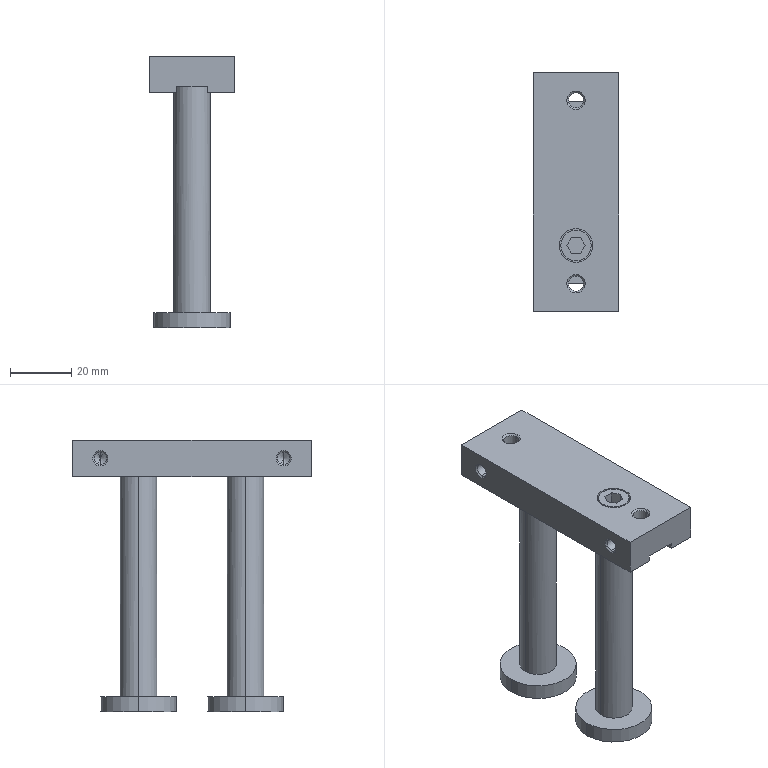Part | STEP file | CXSM25-30(0_0)_ROD_HI | 1 solid | 90 faces | box 28 x 78 x 89 mm | volume 45235 mm3 | plane 38 | cylinder 28 | cone 24 | commonest cylinder face diameters 4.134 x8 4.917 x4 12 x4 25 x4 7 x2 8 x2